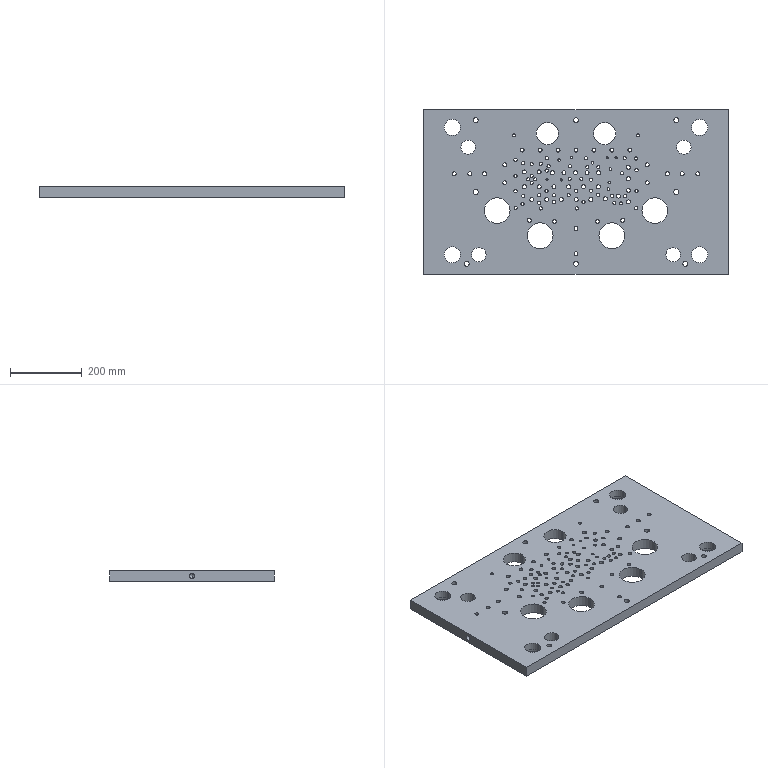Part | SolidWorks | features BaseBody 1 | 1 solid | 622 faces | box 850 x 460 x 30 mm | volume 10345639 mm3 | cylinder 489 | plane 129 | cone 4 | commonest cylinder face diameters 14 x119 11 x104 16 x98 9 x94 6 x10 7 x10